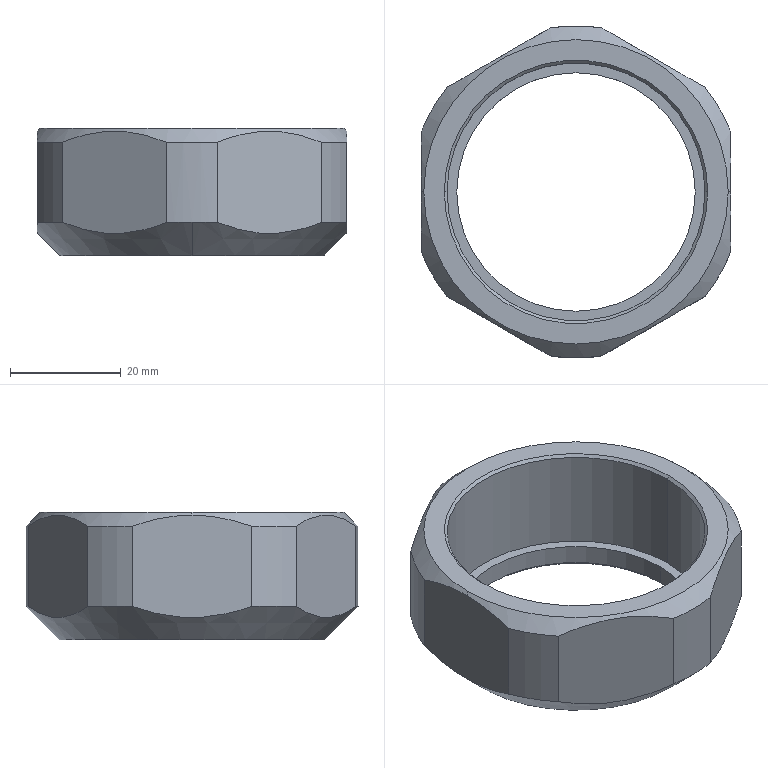Part | SolidWorks | features BaseBody 1 | 1 solid | 27 faces | box 56 x 60 x 23 mm | volume 20223 mm3 | cylinder 10 | plane 9 | cone 8 | commonest cylinder face diameters 60 x6 43.1 x2 46.6 x2
STEP:
#1=CARTESIAN_POINT('',(-23.3,0.,4.));
#2=VERTEX_POINT('',#1);
#3=CARTESIAN_POINT('',(23.3,0.,4.));
#4=VERTEX_POINT('',#3);
#5=CARTESIAN_POINT('',(0.,0.,4.));
#6=DIRECTION('',(0.,0.,1.));
#7=DIRECTION('',(1.,0.,0.));
#8=AXIS2_PLACEMENT_3D('',#5,#6,#7);
#9=CIRCLE('',#8,23.3);
#10=EDGE_CURVE('',#2,#4,#9,.T.);
#11=ORIENTED_EDGE('',*,*,#10,.F.);
#12=CARTESIAN_POINT('',(-23.3,0.,22.5));
#13=VERTEX_POINT('',#12);
#14=CARTESIAN_POINT('',(-23.3,0.,4.));
#15=DIRECTION('',(0.,0.,1.));
#16=VECTOR('',#15,1000.);
#17=LINE('',#14,#16);
#18=EDGE_CURVE('',#2,#13,#17,.T.);
#19=ORIENTED_EDGE('',*,*,#18,.T.);
#20=CARTESIAN_POINT('',(23.3,0.,22.5));
#21=VERTEX_POINT('',#20);
#22=CARTESIAN_POINT('',(0.,0.,22.5));
#23=DIRECTION('',(0.,0.,-1.));
#24=DIRECTION('',(1.,0.,0.));
#25=AXIS2_PLACEMENT_3D('',#22,#23,#24);
#26=CIRCLE('',#25,23.3);
#27=EDGE_CURVE('',#21,#13,#26,.T.);
#28=ORIENTED_EDGE('',*,*,#27,.F.);
#29=CARTESIAN_POINT('',(23.3,0.,4.));
#30=DIRECTION('',(0.,0.,1.));
#31=VECTOR('',#30,1000.);
#32=LINE('',#29,#31);
#33=EDGE_CURVE('',#4,#21,#32,.T.);
#34=ORIENTED_EDGE('',*,*,#33,.F.);
#35=EDGE_LOOP('',(#11,#19,#28,#34));
#36=FACE_OUTER_BOUND('',#35,.T.);
#37=CARTESIAN_POINT('',(0.,0.,4.));
#38=DIRECTION('',(0.,0.,1.));
#39=DIRECTION('',(1.,0.,0.));
#40=AXIS2_PLACEMENT_3D('',#37,#38,#39);
#41=CYLINDRICAL_SURFACE('',#40,23.3);
#42=ADVANCED_FACE('',(#36),#41,.F.);
#43=ORIENTED_EDGE('',*,*,#27,.T.);
#44=CARTESIAN_POINT('',(-23.8,0.,23.));
#45=VERTEX_POINT('',#44);
#46=CARTESIAN_POINT('',(-23.8,0.,23.));
#47=DIRECTION('',(-0.7071,0.,0.7071));
#48=VECTOR('',#47,1000.);
#49=LINE('',#46,#48);
#50=EDGE_CURVE('',#13,#45,#49,.T.);
#51=ORIENTED_EDGE('',*,*,#50,.T.);
#52=CARTESIAN_POINT('',(23.8,0.,23.));
#53=VERTEX_POINT('',#52);
#54=CARTESIAN_POINT('',(0.,0.,23.));
#55=DIRECTION('',(0.,0.,-1.));
#56=DIRECTION('',(1.,0.,0.));
#57=AXIS2_PLACEMENT_3D('',#54,#55,#56);
#58=CIRCLE('',#57,23.8);
#59=EDGE_CURVE('',#53,#45,#58,.T.);
#60=ORIENTED_EDGE('',*,*,#59,.F.);
#61=CARTESIAN_POINT('',(23.8,0.,23.));
#62=DIRECTION('',(0.7071,0.,0.7071));
#63=VECTOR('',#62,1000.);
#64=LINE('',#61,#63);
#65=EDGE_CURVE('',#21,#53,#64,.T.);
#66=ORIENTED_EDGE('',*,*,#65,.F.);
#67=EDGE_LOOP('',(#43,#51,#60,#66));
#68=FACE_OUTER_BOUND('',#67,.T.);
#69=CARTESIAN_POINT('',(0.,0.,23.));
#70=DIRECTION('',(0.,0.,1.));
#71=DIRECTION('',(1.,0.,0.));
#72=AXIS2_PLACEMENT_3D('',#69,#70,#71);
#73=CONICAL_SURFACE('',#72,23.8,0.7854);
#74=ADVANCED_FACE('',(#68),#73,.F.);
#75=CARTESIAN_POINT('',(21.55,0.,4.));
#76=VERTEX_POINT('',#75);
#77=CARTESIAN_POINT('',(-21.55,0.,4.));
#78=VERTEX_POINT('',#77);
#79=CARTESIAN_POINT('',(0.,0.,4.));
#80=DIRECTION('',(0.,0.,-1.));
#81=DIRECTION('',(-1.,0.,0.));
#82=AXIS2_PLACEMENT_3D('',#79,#80,#81);
#83=CIRCLE('',#82,21.55);
#84=EDGE_CURVE('',#76,#78,#83,.T.);
#85=ORIENTED_EDGE('',*,*,#84,.F.);
#86=CARTESIAN_POINT('',(21.55,0.,0.5));
#87=VERTEX_POINT('',#86);
#88=CARTESIAN_POINT('',(21.55,0.,23.));
#89=DIRECTION('',(0.,0.,-1.));
#90=VECTOR('',#89,1000.);
#91=LINE('',#88,#90);
#92=EDGE_CURVE('',#76,#87,#91,.T.);
#93=ORIENTED_EDGE('',*,*,#92,.T.);
#94=CARTESIAN_POINT('',(-21.55,0.,0.5));
#95=VERTEX_POINT('',#94);
#96=CARTESIAN_POINT('',(0.,0.,0.5));
#97=DIRECTION('',(0.,0.,1.));
#98=DIRECTION('',(-1.,0.,0.));
#99=AXIS2_PLACEMENT_3D('',#96,#97,#98);
#100=CIRCLE('',#99,21.55);
#101=EDGE_CURVE('',#95,#87,#100,.T.);
#102=ORIENTED_EDGE('',*,*,#101,.F.);
#103=CARTESIAN_POINT('',(-21.55,0.,23.));
#104=DIRECTION('',(0.,0.,-1.));
#105=VECTOR('',#104,1000.);
#106=LINE('',#103,#105);
#107=EDGE_CURVE('',#78,#95,#106,.T.);
#108=ORIENTED_EDGE('',*,*,#107,.F.);
#109=EDGE_LOOP('',(#85,#93,#102,#108));
#110=FACE_OUTER_BOUND('',#109,.T.);
#111=CARTESIAN_POINT('',(0.,0.,23.));
#112=DIRECTION('',(0.,0.,-1.));
#113=DIRECTION('',(-1.,0.,0.));
#114=AXIS2_PLACEMENT_3D('',#111,#112,#113);
#115=CYLINDRICAL_SURFACE('',#114,21.55);
#116=ADVANCED_FACE('',(#110),#115,.F.);
#117=ORIENTED_EDGE('',*,*,#101,.T.);
#118=CARTESIAN_POINT('',(22.05,0.,0.));
#119=VERTEX_POINT('',#118);
#120=CARTESIAN_POINT('',(22.05,0.,0.));
#121=DIRECTION('',(0.7071,0.,-0.7071));
#122=VECTOR('',#121,1000.);
#123=LINE('',#120,#122);
#124=EDGE_CURVE('',#87,#119,#123,.T.);
#125=ORIENTED_EDGE('',*,*,#124,.T.);
#126=CARTESIAN_POINT('',(-22.05,0.,0.));
#127=VERTEX_POINT('',#126);
#128=CARTESIAN_POINT('',(0.,0.,0.));
#129=DIRECTION('',(0.,0.,1.));
#130=DIRECTION('',(-1.,0.,0.));
#131=AXIS2_PLACEMENT_3D('',#128,#129,#130);
#132=CIRCLE('',#131,22.05);
#133=EDGE_CURVE('',#127,#119,#132,.T.);
#134=ORIENTED_EDGE('',*,*,#133,.F.);
#135=CARTESIAN_POINT('',(-22.05,0.,0.));
#136=DIRECTION('',(-0.7071,0.,-0.7071));
#137=VECTOR('',#136,1000.);
#138=LINE('',#135,#137);
#139=EDGE_CURVE('',#95,#127,#138,.T.);
#140=ORIENTED_EDGE('',*,*,#139,.F.);
#141=EDGE_LOOP('',(#117,#125,#134,#140));
#142=FACE_OUTER_BOUND('',#141,.T.);
#143=CARTESIAN_POINT('',(0.,0.,0.));
#144=DIRECTION('',(0.,0.,-1.));
#145=DIRECTION('',(-1.,0.,0.));
#146=AXIS2_PLACEMENT_3D('',#143,#144,#145);
#147=CONICAL_SURFACE('',#146,22.05,0.7854);
#148=ADVANCED_FACE('',(#142),#147,.F.);
#149=CARTESIAN_POINT('',(27.5,0.,23.));
#150=VERTEX_POINT('',#149);
#151=CARTESIAN_POINT('',(-27.5,0.,23.));
#152=VERTEX_POINT('',#151);
#153=CARTESIAN_POINT('',(0.,0.,23.));
#154=DIRECTION('',(0.,0.,1.));
#155=DIRECTION('',(-1.,0.,0.));
#156=AXIS2_PLACEMENT_3D('',#153,#154,#155);
#157=CIRCLE('',#156,27.5);
#158=EDGE_CURVE('',#150,#152,#157,.T.);
#159=ORIENTED_EDGE('',*,*,#158,.F.);
#160=CARTESIAN_POINT('',(28.,0.,22.5));
#161=VERTEX_POINT('',#160);
#162=CARTESIAN_POINT('',(30.,0.,20.5));
#163=DIRECTION('',(0.7071,0.,-0.7071));
#164=VECTOR('',#163,1000.);
#165=LINE('',#162,#164);
#166=EDGE_CURVE('',#150,#161,#165,.T.);
#167=ORIENTED_EDGE('',*,*,#166,.T.);
#168=CARTESIAN_POINT('',(28.,10.77,20.5));
#169=VERTEX_POINT('',#168);
#170=CARTESIAN_POINT('',(28.,0.,22.5));
#171=CARTESIAN_POINT('',(28.,1.857,22.5));
#172=CARTESIAN_POINT('',(28.,3.679,22.314));
#173=CARTESIAN_POINT('',(28.,7.266,21.626));
#174=CARTESIAN_POINT('',(28.,9.029,21.125));
#175=CARTESIAN_POINT('',(28.,10.77,20.5));
#176=B_SPLINE_CURVE_WITH_KNOTS('',3,(#170,#171,#172,#173,#174,#175),.UNSPECIFIED.,.F.,.F.,(4,2,4),(0.,0.005477,0.01095),.UNSPECIFIED.);
#177=EDGE_CURVE('',#161,#169,#176,.T.);
#178=ORIENTED_EDGE('',*,*,#177,.T.);
#179=CARTESIAN_POINT('',(23.327,18.864,20.5));
#180=VERTEX_POINT('',#179);
#181=CARTESIAN_POINT('',(0.,0.,20.5));
#182=DIRECTION('',(0.,0.,1.));
#183=DIRECTION('',(-1.,0.,0.));
#184=AXIS2_PLACEMENT_3D('',#181,#182,#183);
#185=CIRCLE('',#184,30.);
#186=EDGE_CURVE('',#169,#180,#185,.T.);
#187=ORIENTED_EDGE('',*,*,#186,.T.);
#188=CARTESIAN_POINT('',(4.673,29.634,20.5));
#189=VERTEX_POINT('',#188);
#190=CARTESIAN_POINT('',(23.327,18.864,20.5));
#191=CARTESIAN_POINT('',(21.82,19.734,21.125));
#192=CARTESIAN_POINT('',(20.292,20.616,21.626));
#193=CARTESIAN_POINT('',(17.186,22.409,22.314));
#194=CARTESIAN_POINT('',(15.608,23.32,22.5));
#195=CARTESIAN_POINT('',(12.392,25.177,22.5));
#196=CARTESIAN_POINT('',(10.813,26.088,22.314));
#197=CARTESIAN_POINT('',(7.708,27.882,21.626));
#198=CARTESIAN_POINT('',(6.18,28.763,21.125));
#199=CARTESIAN_POINT('',(4.673,29.634,20.5));
#200=B_SPLINE_CURVE_WITH_KNOTS('',3,(#190,#191,#192,#193,#194,#195,#196,#197,#198,#199),.UNSPECIFIED.,.F.,.F.,(4,2,2,2,4),(-0.01095,-0.005472,0.000005126,0.005482,0.01096),.UNSPECIFIED.);
#201=EDGE_CURVE('',#180,#189,#200,.T.);
#202=ORIENTED_EDGE('',*,*,#201,.T.);
#203=CARTESIAN_POINT('',(-4.673,29.634,20.5));
#204=VERTEX_POINT('',#203);
#205=CARTESIAN_POINT('',(0.,0.,20.5));
#206=DIRECTION('',(0.,0.,1.));
#207=DIRECTION('',(-1.,0.,0.));
#208=AXIS2_PLACEMENT_3D('',#205,#206,#207);
#209=CIRCLE('',#208,30.);
#210=EDGE_CURVE('',#189,#204,#209,.T.);
#211=ORIENTED_EDGE('',*,*,#210,.T.);
#212=CARTESIAN_POINT('',(-23.327,18.864,20.5));
#213=VERTEX_POINT('',#212);
#214=CARTESIAN_POINT('',(-4.673,29.634,20.5));
#215=CARTESIAN_POINT('',(-6.18,28.763,21.125));
#216=CARTESIAN_POINT('',(-7.708,27.881,21.626));
#217=CARTESIAN_POINT('',(-10.814,26.088,22.314));
#218=CARTESIAN_POINT('',(-12.392,25.177,22.5));
#219=CARTESIAN_POINT('',(-15.608,23.32,22.5));
#220=CARTESIAN_POINT('',(-17.187,22.409,22.314));
#221=CARTESIAN_POINT('',(-20.292,20.616,21.626));
#222=CARTESIAN_POINT('',(-21.82,19.734,21.125));
#223=CARTESIAN_POINT('',(-23.327,18.864,20.5));
#224=B_SPLINE_CURVE_WITH_KNOTS('',3,(#214,#215,#216,#217,#218,#219,#220,#221,#222,#223),.UNSPECIFIED.,.F.,.F.,(4,2,2,2,4),(-0.01095,-0.005472,0.000005126,0.005482,0.01096),.UNSPECIFIED.);
#225=EDGE_CURVE('',#204,#213,#224,.T.);
#226=ORIENTED_EDGE('',*,*,#225,.T.);
#227=CARTESIAN_POINT('',(-28.,10.77,20.5));
#228=VERTEX_POINT('',#227);
#229=CARTESIAN_POINT('',(0.,0.,20.5));
#230=DIRECTION('',(0.,0.,1.));
#231=DIRECTION('',(-1.,0.,0.));
#232=AXIS2_PLACEMENT_3D('',#229,#230,#231);
#233=CIRCLE('',#232,30.);
#234=EDGE_CURVE('',#213,#228,#233,.T.);
#235=ORIENTED_EDGE('',*,*,#234,.T.);
#236=CARTESIAN_POINT('',(-28.,0.,22.5));
#237=VERTEX_POINT('',#236);
#238=CARTESIAN_POINT('',(-28.,10.77,20.5));
#239=CARTESIAN_POINT('',(-28.,9.029,21.125));
#240=CARTESIAN_POINT('',(-28.,7.266,21.626));
#241=CARTESIAN_POINT('',(-28.,3.679,22.314));
#242=CARTESIAN_POINT('',(-28.,1.857,22.5));
#243=CARTESIAN_POINT('',(-28.,0.,22.5));
#244=B_SPLINE_CURVE_WITH_KNOTS('',3,(#238,#239,#240,#241,#242,#243),.UNSPECIFIED.,.F.,.F.,(4,2,4),(0.,0.005477,0.01095),.UNSPECIFIED.);
#245=EDGE_CURVE('',#228,#237,#244,.T.);
#246=ORIENTED_EDGE('',*,*,#245,.T.);
#247=CARTESIAN_POINT('',(-30.,0.,20.5));
#248=DIRECTION('',(-0.7071,0.,-0.7071));
#249=VECTOR('',#248,1000.);
#250=LINE('',#247,#249);
#251=EDGE_CURVE('',#152,#237,#250,.T.);
#252=ORIENTED_EDGE('',*,*,#251,.F.);
#253=EDGE_LOOP('',(#159,#167,#178,#187,#202,#211,#226,#235,#246,#252));
#254=FACE_OUTER_BOUND('',#253,.T.);
#255=CARTESIAN_POINT('',(0.,0.,20.5));
#256=DIRECTION('',(0.,0.,-1.));
#257=DIRECTION('',(-1.,0.,0.));
#258=AXIS2_PLACEMENT_3D('',#255,#256,#257);
#259=CONICAL_SURFACE('',#258,30.,0.7854);
#260=ADVANCED_FACE('',(#254),#259,.T.);
#261=CARTESIAN_POINT('',(0.,-24.,0.));
#262=VERTEX_POINT('',#261);
#263=CARTESIAN_POINT('',(0.,24.,0.));
#264=VERTEX_POINT('',#263);
#265=CARTESIAN_POINT('',(0.,0.,0.));
#266=DIRECTION('',(0.,0.,1.));
#267=DIRECTION('',(0.,-1.,0.));
#268=AXIS2_PLACEMENT_3D('',#265,#266,#267);
#269=CIRCLE('',#268,24.);
#270=EDGE_CURVE('',#262,#264,#269,.T.);
#271=ORIENTED_EDGE('',*,*,#270,.T.);
#272=CARTESIAN_POINT('',(0.,30.,6.));
#273=VERTEX_POINT('',#272);
#274=CARTESIAN_POINT('',(0.,30.,6.));
#275=DIRECTION('',(0.,0.7071,0.7071));
#276=VECTOR('',#275,1000.);
#277=LINE('',#274,#276);
#278=EDGE_CURVE('',#264,#273,#277,.T.);
#279=ORIENTED_EDGE('',*,*,#278,.T.);
#280=CARTESIAN_POINT('',(4.673,29.634,6.));
#281=VERTEX_POINT('',#280);
#282=CARTESIAN_POINT('',(0.,0.,6.));
#283=DIRECTION('',(0.,0.,1.));
#284=DIRECTION('',(-1.,0.,0.));
#285=AXIS2_PLACEMENT_3D('',#282,#283,#284);
#286=CIRCLE('',#285,30.);
#287=EDGE_CURVE('',#281,#273,#286,.T.);
#288=ORIENTED_EDGE('',*,*,#287,.F.);
#289=CARTESIAN_POINT('',(23.327,18.864,6.));
#290=VERTEX_POINT('',#289);
#291=CARTESIAN_POINT('',(4.673,29.634,6.));
#292=CARTESIAN_POINT('',(6.18,28.763,5.375));
#293=CARTESIAN_POINT('',(7.708,27.882,4.874));
#294=CARTESIAN_POINT('',(10.813,26.088,4.186));
#295=CARTESIAN_POINT('',(12.392,25.177,4.));
#296=CARTESIAN_POINT('',(15.608,23.32,4.));
#297=CARTESIAN_POINT('',(17.186,22.409,4.186));
#298=CARTESIAN_POINT('',(20.292,20.616,4.874));
#299=CARTESIAN_POINT('',(21.82,19.734,5.375));
#300=CARTESIAN_POINT('',(23.327,18.864,6.));
#301=B_SPLINE_CURVE_WITH_KNOTS('',3,(#291,#292,#293,#294,#295,#296,#297,#298,#299,#300),.UNSPECIFIED.,.F.,.F.,(4,2,2,2,4),(-0.01096,-0.005482,-0.000005126,0.005472,0.01095),.UNSPECIFIED.);
#302=EDGE_CURVE('',#281,#290,#301,.T.);
#303=ORIENTED_EDGE('',*,*,#302,.T.);
#304=CARTESIAN_POINT('',(28.,10.77,6.));
#305=VERTEX_POINT('',#304);
#306=CARTESIAN_POINT('',(0.,0.,6.));
#307=DIRECTION('',(0.,0.,1.));
#308=DIRECTION('',(-1.,0.,0.));
#309=AXIS2_PLACEMENT_3D('',#306,#307,#308);
#310=CIRCLE('',#309,30.);
#311=EDGE_CURVE('',#305,#290,#310,.T.);
#312=ORIENTED_EDGE('',*,*,#311,.F.);
#313=CARTESIAN_POINT('',(28.,-10.77,6.));
#314=VERTEX_POINT('',#313);
#315=CARTESIAN_POINT('',(28.,10.77,6.));
#316=CARTESIAN_POINT('',(28.,9.029,5.375));
#317=CARTESIAN_POINT('',(28.,7.266,4.874));
#318=CARTESIAN_POINT('',(28.,3.679,4.186));
#319=CARTESIAN_POINT('',(28.,1.857,4.));
#320=CARTESIAN_POINT('',(28.,-1.857,4.));
#321=CARTESIAN_POINT('',(28.,-3.679,4.186));
#322=CARTESIAN_POINT('',(28.,-7.266,4.874));
#323=CARTESIAN_POINT('',(28.,-9.029,5.375));
#324=CARTESIAN_POINT('',(28.,-10.77,6.));
#325=B_SPLINE_CURVE_WITH_KNOTS('',3,(#315,#316,#317,#318,#319,#320,#321,#322,#323,#324),.UNSPECIFIED.,.F.,.F.,(4,2,2,2,4),(-0.01095,-0.005477,0.,0.005477,0.01095),.UNSPECIFIED.);
#326=EDGE_CURVE('',#305,#314,#325,.T.);
#327=ORIENTED_EDGE('',*,*,#326,.T.);
#328=CARTESIAN_POINT('',(23.327,-18.864,6.));
#329=VERTEX_POINT('',#328);
#330=CARTESIAN_POINT('',(0.,0.,6.));
#331=DIRECTION('',(0.,0.,1.));
#332=DIRECTION('',(-1.,0.,0.));
#333=AXIS2_PLACEMENT_3D('',#330,#331,#332);
#334=CIRCLE('',#333,30.);
#335=EDGE_CURVE('',#329,#314,#334,.T.);
#336=ORIENTED_EDGE('',*,*,#335,.F.);
#337=CARTESIAN_POINT('',(4.673,-29.634,6.));
#338=VERTEX_POINT('',#337);
#339=CARTESIAN_POINT('',(23.327,-18.864,6.));
#340=CARTESIAN_POINT('',(21.82,-19.734,5.375));
#341=CARTESIAN_POINT('',(20.292,-20.616,4.874));
#342=CARTESIAN_POINT('',(17.187,-22.409,4.186));
#343=CARTESIAN_POINT('',(15.608,-23.32,4.));
#344=CARTESIAN_POINT('',(12.392,-25.177,4.));
#345=CARTESIAN_POINT('',(10.814,-26.088,4.186));
#346=CARTESIAN_POINT('',(7.708,-27.881,4.874));
#347=CARTESIAN_POINT('',(6.18,-28.763,5.375));
#348=CARTESIAN_POINT('',(4.673,-29.634,6.));
#349=B_SPLINE_CURVE_WITH_KNOTS('',3,(#339,#340,#341,#342,#343,#344,#345,#346,#347,#348),.UNSPECIFIED.,.F.,.F.,(4,2,2,2,4),(-0.01096,-0.005482,-0.000005126,0.005472,0.01095),.UNSPECIFIED.);
#350=EDGE_CURVE('',#329,#338,#349,.T.);
#351=ORIENTED_EDGE('',*,*,#350,.T.);
#352=CARTESIAN_POINT('',(0.,-30.,6.));
#353=VERTEX_POINT('',#352);
#354=CARTESIAN_POINT('',(0.,0.,6.));
#355=DIRECTION('',(0.,0.,1.));
#356=DIRECTION('',(-1.,0.,0.));
#357=AXIS2_PLACEMENT_3D('',#354,#355,#356);
#358=CIRCLE('',#357,30.);
#359=EDGE_CURVE('',#353,#338,#358,.T.);
#360=ORIENTED_EDGE('',*,*,#359,.F.);
#361=CARTESIAN_POINT('',(0.,-30.,6.));
#362=DIRECTION('',(0.,-0.7071,0.7071));
#363=VECTOR('',#362,1000.);
#364=LINE('',#361,#363);
#365=EDGE_CURVE('',#262,#353,#364,.T.);
#366=ORIENTED_EDGE('',*,*,#365,.F.);
#367=EDGE_LOOP('',(#271,#279,#288,#303,#312,#327,#336,#351,#360,#366));
#368=FACE_OUTER_BOUND('',#367,.T.);
#369=CARTESIAN_POINT('',(0.,0.,6.));
#370=DIRECTION('',(0.,0.,1.));
#371=DIRECTION('',(0.,-1.,0.));
#372=AXIS2_PLACEMENT_3D('',#369,#370,#371);
#373=CONICAL_SURFACE('',#372,30.,0.7854);
#374=ADVANCED_FACE('',(#368),#373,.T.);
#375=ORIENTED_EDGE('',*,*,#18,.F.);
#376=CARTESIAN_POINT('',(0.,0.,4.));
#377=DIRECTION('',(0.,0.,1.));
#378=DIRECTION('',(1.,0.,0.));
#379=AXIS2_PLACEMENT_3D('',#376,#377,#378);
#380=CIRCLE('',#379,23.3);
#381=EDGE_CURVE('',#4,#2,#380,.T.);
#382=ORIENTED_EDGE('',*,*,#381,.F.);
#383=ORIENTED_EDGE('',*,*,#33,.T.);
#384=CARTESIAN_POINT('',(0.,0.,22.5));
#385=DIRECTION('',(0.,0.,-1.));
#386=DIRECTION('',(1.,0.,0.));
#387=AXIS2_PLACEMENT_3D('',#384,#385,#386);
#388=CIRCLE('',#387,23.3);
#389=EDGE_CURVE('',#13,#21,#388,.T.);
#390=ORIENTED_EDGE('',*,*,#389,.F.);
#391=EDGE_LOOP('',(#375,#382,#383,#390));
#392=FACE_OUTER_BOUND('',#391,.T.);
#393=CARTESIAN_POINT('',(0.,0.,4.));
#394=DIRECTION('',(0.,0.,1.));
#395=DIRECTION('',(1.,0.,0.));
#396=AXIS2_PLACEMENT_3D('',#393,#394,#395);
#397=CYLINDRICAL_SURFACE('',#396,23.3);
#398=ADVANCED_FACE('',(#392),#397,.F.);
#399=CARTESIAN_POINT('',(0.,0.,4.));
#400=DIRECTION('',(0.,0.,-1.));
#401=DIRECTION('',(-1.,0.,0.));
#402=AXIS2_PLACEMENT_3D('',#399,#400,#401);
#403=CIRCLE('',#402,21.55);
#404=EDGE_CURVE('',#78,#76,#403,.T.);
#405=ORIENTED_EDGE('',*,*,#404,.T.);
#406=ORIENTED_EDGE('',*,*,#84,.T.);
#407=EDGE_LOOP('',(#405,#406));
#408=FACE_BOUND('',#407,.T.);
#409=ORIENTED_EDGE('',*,*,#381,.T.);
#410=ORIENTED_EDGE('',*,*,#10,.T.);
#411=EDGE_LOOP('',(#409,#410));
#412=FACE_OUTER_BOUND('',#411,.T.);
#413=CARTESIAN_POINT('',(0.,0.,4.));
#414=DIRECTION('',(0.,0.,1.));
#415=DIRECTION('',(1.,0.,0.));
#416=AXIS2_PLACEMENT_3D('',#413,#414,#415);
#417=PLANE('',#416);
#418=ADVANCED_FACE('',(#408,#412),#417,.T.);
#419=ORIENTED_EDGE('',*,*,#50,.F.);
#420=ORIENTED_EDGE('',*,*,#389,.T.);
#421=ORIENTED_EDGE('',*,*,#65,.T.);
#422=CARTESIAN_POINT('',(0.,0.,23.));
#423=DIRECTION('',(0.,0.,-1.));
#424=DIRECTION('',(1.,0.,0.));
#425=AXIS2_PLACEMENT_3D('',#422,#423,#424);
#426=CIRCLE('',#425,23.8);
#427=EDGE_CURVE('',#45,#53,#426,.T.);
#428=ORIENTED_EDGE('',*,*,#427,.F.);
#429=EDGE_LOOP('',(#419,#420,#421,#428));
#430=FACE_OUTER_BOUND('',#429,.T.);
#431=CARTESIAN_POINT('',(0.,0.,23.));
#432=DIRECTION('',(0.,0.,1.));
#433=DIRECTION('',(1.,0.,0.));
#434=AXIS2_PLACEMENT_3D('',#431,#432,#433);
#435=CONICAL_SURFACE('',#434,23.8,0.7854);
#436=ADVANCED_FACE('',(#430),#435,.F.);
#437=ORIENTED_EDGE('',*,*,#92,.F.);
#438=ORIENTED_EDGE('',*,*,#404,.F.);
#439=ORIENTED_EDGE('',*,*,#107,.T.);
#440=CARTESIAN_POINT('',(0.,0.,0.5));
#441=DIRECTION('',(0.,0.,1.));
#442=DIRECTION('',(-1.,0.,0.));
#443=AXIS2_PLACEMENT_3D('',#440,#441,#442);
#444=CIRCLE('',#443,21.55);
#445=EDGE_CURVE('',#87,#95,#444,.T.);
#446=ORIENTED_EDGE('',*,*,#445,.F.);
#447=EDGE_LOOP('',(#437,#438,#439,#446));
#448=FACE_OUTER_BOUND('',#447,.T.);
#449=CARTESIAN_POINT('',(0.,0.,23.));
#450=DIRECTION('',(0.,0.,-1.));
#451=DIRECTION('',(-1.,0.,0.));
#452=AXIS2_PLACEMENT_3D('',#449,#450,#451);
#453=CYLINDRICAL_SURFACE('',#452,21.55);
#454=ADVANCED_FACE('',(#448),#453,.F.);
#455=ORIENTED_EDGE('',*,*,#59,.T.);
#456=ORIENTED_EDGE('',*,*,#427,.T.);
#457=EDGE_LOOP('',(#455,#456));
#458=FACE_BOUND('',#457,.T.);
#459=CARTESIAN_POINT('',(0.,0.,23.));
#460=DIRECTION('',(0.,0.,1.));
#461=DIRECTION('',(-1.,0.,0.));
#462=AXIS2_PLACEMENT_3D('',#459,#460,#461);
#463=CIRCLE('',#462,27.5);
#464=EDGE_CURVE('',#152,#150,#463,.T.);
#465=ORIENTED_EDGE('',*,*,#464,.T.);
#466=ORIENTED_EDGE('',*,*,#158,.T.);
#467=EDGE_LOOP('',(#465,#466));
#468=FACE_OUTER_BOUND('',#467,.T.);
#469=CARTESIAN_POINT('',(0.,0.,23.));
#470=DIRECTION('',(0.,0.,1.));
#471=DIRECTION('',(1.,0.,0.));
#472=AXIS2_PLACEMENT_3D('',#469,#470,#471);
#473=PLANE('',#472);
#474=ADVANCED_FACE('',(#458,#468),#473,.T.);
#475=ORIENTED_EDGE('',*,*,#124,.F.);
#476=ORIENTED_EDGE('',*,*,#445,.T.);
#477=ORIENTED_EDGE('',*,*,#139,.T.);
#478=CARTESIAN_POINT('',(0.,0.,0.));
#479=DIRECTION('',(0.,0.,1.));
#480=DIRECTION('',(-1.,0.,0.));
#481=AXIS2_PLACEMENT_3D('',#478,#479,#480);
#482=CIRCLE('',#481,22.05);
#483=EDGE_CURVE('',#119,#127,#482,.T.);
#484=ORIENTED_EDGE('',*,*,#483,.F.);
#485=EDGE_LOOP('',(#475,#476,#477,#484));
#486=FACE_OUTER_BOUND('',#485,.T.);
#487=CARTESIAN_POINT('',(0.,0.,0.));
#488=DIRECTION('',(0.,0.,-1.));
#489=DIRECTION('',(-1.,0.,0.));
#490=AXIS2_PLACEMENT_3D('',#487,#488,#489);
#491=CONICAL_SURFACE('',#490,22.05,0.7854);
#492=ADVANCED_FACE('',(#486),#491,.F.);
#493=ORIENTED_EDGE('',*,*,#166,.F.);
#494=ORIENTED_EDGE('',*,*,#464,.F.);
#495=ORIENTED_EDGE('',*,*,#251,.T.);
#496=CARTESIAN_POINT('',(-28.,-10.77,20.5));
#497=VERTEX_POINT('',#496);
#498=CARTESIAN_POINT('',(-28.,0.,22.5));
#499=CARTESIAN_POINT('',(-28.,-1.857,22.5));
#500=CARTESIAN_POINT('',(-28.,-3.679,22.314));
#501=CARTESIAN_POINT('',(-28.,-7.266,21.626));
#502=CARTESIAN_POINT('',(-28.,-9.029,21.125));
#503=CARTESIAN_POINT('',(-28.,-10.77,20.5));
#504=B_SPLINE_CURVE_WITH_KNOTS('',3,(#498,#499,#500,#501,#502,#503),.UNSPECIFIED.,.F.,.F.,(4,2,4),(0.01095,0.01643,0.02191),.UNSPECIFIED.);
#505=EDGE_CURVE('',#237,#497,#504,.T.);
#506=ORIENTED_EDGE('',*,*,#505,.T.);
#507=CARTESIAN_POINT('',(-23.327,-18.864,20.5));
#508=VERTEX_POINT('',#507);
#509=CARTESIAN_POINT('',(0.,0.,20.5));
#510=DIRECTION('',(0.,0.,1.));
#511=DIRECTION('',(1.,0.,0.));
#512=AXIS2_PLACEMENT_3D('',#509,#510,#511);
#513=CIRCLE('',#512,30.);
#514=EDGE_CURVE('',#497,#508,#513,.T.);
#515=ORIENTED_EDGE('',*,*,#514,.T.);
#516=CARTESIAN_POINT('',(-4.673,-29.634,20.5));
#517=VERTEX_POINT('',#516);
#518=CARTESIAN_POINT('',(-23.327,-18.864,20.5));
#519=CARTESIAN_POINT('',(-21.82,-19.734,21.125));
#520=CARTESIAN_POINT('',(-20.292,-20.616,21.626));
#521=CARTESIAN_POINT('',(-17.186,-22.409,22.314));
#522=CARTESIAN_POINT('',(-15.608,-23.32,22.5));
#523=CARTESIAN_POINT('',(-12.392,-25.177,22.5));
#524=CARTESIAN_POINT('',(-10.813,-26.088,22.314));
#525=CARTESIAN_POINT('',(-7.708,-27.882,21.626));
#526=CARTESIAN_POINT('',(-6.18,-28.763,21.125));
#527=CARTESIAN_POINT('',(-4.673,-29.634,20.5));
#528=B_SPLINE_CURVE_WITH_KNOTS('',3,(#518,#519,#520,#521,#522,#523,#524,#525,#526,#527),.UNSPECIFIED.,.F.,.F.,(4,2,2,2,4),(-0.01095,-0.005472,0.000005126,0.005482,0.01096),.UNSPECIFIED.);
#529=EDGE_CURVE('',#508,#517,#528,.T.);
#530=ORIENTED_EDGE('',*,*,#529,.T.);
#531=CARTESIAN_POINT('',(4.673,-29.634,20.5));
#532=VERTEX_POINT('',#531);
#533=CARTESIAN_POINT('',(0.,0.,20.5));
#534=DIRECTION('',(0.,0.,1.));
#535=DIRECTION('',(1.,0.,0.));
#536=AXIS2_PLACEMENT_3D('',#533,#534,#535);
#537=CIRCLE('',#536,30.);
#538=EDGE_CURVE('',#517,#532,#537,.T.);
#539=ORIENTED_EDGE('',*,*,#538,.T.);
#540=CARTESIAN_POINT('',(23.327,-18.864,20.5));
#541=VERTEX_POINT('',#540);
#542=CARTESIAN_POINT('',(4.673,-29.634,20.5));
#543=CARTESIAN_POINT('',(6.18,-28.763,21.125));
#544=CARTESIAN_POINT('',(7.708,-27.881,21.626));
#545=CARTESIAN_POINT('',(10.814,-26.088,22.314));
#546=CARTESIAN_POINT('',(12.392,-25.177,22.5));
#547=CARTESIAN_POINT('',(15.608,-23.32,22.5));
#548=CARTESIAN_POINT('',(17.187,-22.409,22.314));
#549=CARTESIAN_POINT('',(20.292,-20.616,21.626));
#550=CARTESIAN_POINT('',(21.82,-19.734,21.125));
#551=CARTESIAN_POINT('',(23.327,-18.864,20.5));
#552=B_SPLINE_CURVE_WITH_KNOTS('',3,(#542,#543,#544,#545,#546,#547,#548,#549,#550,#551),.UNSPECIFIED.,.F.,.F.,(4,2,2,2,4),(-0.01095,-0.005472,0.000005126,0.005482,0.01096),.UNSPECIFIED.);
#553=EDGE_CURVE('',#532,#541,#552,.T.);
#554=ORIENTED_EDGE('',*,*,#553,.T.);
#555=CARTESIAN_POINT('',(28.,-10.77,20.5));
#556=VERTEX_POINT('',#555);
#557=CARTESIAN_POINT('',(0.,0.,20.5));
#558=DIRECTION('',(0.,0.,1.));
#559=DIRECTION('',(1.,0.,0.));
#560=AXIS2_PLACEMENT_3D('',#557,#558,#559);
#561=CIRCLE('',#560,30.);
#562=EDGE_CURVE('',#541,#556,#561,.T.);
#563=ORIENTED_EDGE('',*,*,#562,.T.);
#564=CARTESIAN_POINT('',(28.,-10.77,20.5));
#565=CARTESIAN_POINT('',(28.,-9.029,21.125));
#566=CARTESIAN_POINT('',(28.,-7.266,21.626));
#567=CARTESIAN_POINT('',(28.,-3.679,22.314));
#568=CARTESIAN_POINT('',(28.,-1.857,22.5));
#569=CARTESIAN_POINT('',(28.,0.,22.5));
#570=B_SPLINE_CURVE_WITH_KNOTS('',3,(#564,#565,#566,#567,#568,#569),.UNSPECIFIED.,.F.,.F.,(4,2,4),(-0.01095,-0.005477,0.),.UNSPECIFIED.);
#571=EDGE_CURVE('',#556,#161,#570,.T.);
#572=ORIENTED_EDGE('',*,*,#571,.T.);
#573=EDGE_LOOP('',(#493,#494,#495,#506,#515,#530,#539,#554,#563,#572));
#574=FACE_OUTER_BOUND('',#573,.T.);
#575=CARTESIAN_POINT('',(0.,0.,20.5));
#576=DIRECTION('',(0.,0.,-1.));
#577=DIRECTION('',(-1.,0.,0.));
#578=AXIS2_PLACEMENT_3D('',#575,#576,#577);
#579=CONICAL_SURFACE('',#578,30.,0.7854);
#580=ADVANCED_FACE('',(#574),#579,.T.);
#581=ORIENTED_EDGE('',*,*,#133,.T.);
#582=ORIENTED_EDGE('',*,*,#483,.T.);
#583=EDGE_LOOP('',(#581,#582));
#584=FACE_BOUND('',#583,.T.);
#585=ORIENTED_EDGE('',*,*,#270,.F.);
#586=CARTESIAN_POINT('',(0.,0.,0.));
#587=DIRECTION('',(0.,0.,1.));
#588=DIRECTION('',(0.,-1.,0.));
#589=AXIS2_PLACEMENT_3D('',#586,#587,#588);
#590=CIRCLE('',#589,24.);
#591=EDGE_CURVE('',#264,#262,#590,.T.);
#592=ORIENTED_EDGE('',*,*,#591,.F.);
#593=EDGE_LOOP('',(#585,#592));
#594=FACE_OUTER_BOUND('',#593,.T.);
#595=CARTESIAN_POINT('',(0.,0.,0.));
#596=DIRECTION('',(0.,0.,1.));
#597=DIRECTION('',(1.,0.,0.));
#598=AXIS2_PLACEMENT_3D('',#595,#596,#597);
#599=PLANE('',#598);
#600=ADVANCED_FACE('',(#584,#594),#599,.F.);
#601=CARTESIAN_POINT('',(-28.,10.77,6.));
#602=VERTEX_POINT('',#601);
#603=CARTESIAN_POINT('',(-28.,10.77,23.));
#604=DIRECTION('',(0.,0.,1.));
#605=VECTOR('',#604,1000.);
#606=LINE('',#603,#605);
#607=EDGE_CURVE('',#602,#228,#606,.T.);
#608=ORIENTED_EDGE('',*,*,#607,.F.);
#609=CARTESIAN_POINT('',(-28.,-10.77,6.));
#610=VERTEX_POINT('',#609);
#611=CARTESIAN_POINT('',(-28.,-10.77,6.));
#612=CARTESIAN_POINT('',(-28.,-9.029,5.375));
#613=CARTESIAN_POINT('',(-28.,-7.266,4.874));
#614=CARTESIAN_POINT('',(-28.,-3.679,4.186));
#615=CARTESIAN_POINT('',(-28.,-1.857,4.));
#616=CARTESIAN_POINT('',(-28.,1.857,4.));
#617=CARTESIAN_POINT('',(-28.,3.679,4.186));
#618=CARTESIAN_POINT('',(-28.,7.266,4.874));
#619=CARTESIAN_POINT('',(-28.,9.029,5.375));
#620=CARTESIAN_POINT('',(-28.,10.77,6.));
#621=B_SPLINE_CURVE_WITH_KNOTS('',3,(#611,#612,#613,#614,#615,#616,#617,#618,#619,#620),.UNSPECIFIED.,.F.,.F.,(4,2,2,2,4),(-0.01095,-0.005477,0.,0.005477,0.01095),.UNSPECIFIED.);
#622=EDGE_CURVE('',#610,#602,#621,.T.);
#623=ORIENTED_EDGE('',*,*,#622,.F.);
#624=CARTESIAN_POINT('',(-28.,-10.77,23.));
#625=DIRECTION('',(0.,0.,-1.));
#626=VECTOR('',#625,1000.);
#627=LINE('',#624,#626);
#628=EDGE_CURVE('',#497,#610,#627,.T.);
#629=ORIENTED_EDGE('',*,*,#628,.F.);
#630=ORIENTED_EDGE('',*,*,#505,.F.);
#631=ORIENTED_EDGE('',*,*,#245,.F.);
#632=EDGE_LOOP('',(#608,#623,#629,#630,#631));
#633=FACE_OUTER_BOUND('',#632,.T.);
#634=CARTESIAN_POINT('',(-28.,10.77,23.));
#635=DIRECTION('',(1.,0.,0.));
#636=DIRECTION('',(0.,0.,-1.));
#637=AXIS2_PLACEMENT_3D('',#634,#635,#636);
#638=PLANE('',#637);
#639=ADVANCED_FACE('',(#633),#638,.F.);
#640=CARTESIAN_POINT('',(-23.327,18.864,6.));
#641=VERTEX_POINT('',#640);
#642=CARTESIAN_POINT('',(0.,0.,6.));
#643=DIRECTION('',(0.,0.,1.));
#644=DIRECTION('',(-1.,0.,0.));
#645=AXIS2_PLACEMENT_3D('',#642,#643,#644);
#646=CIRCLE('',#645,30.);
#647=EDGE_CURVE('',#641,#602,#646,.T.);
#648=ORIENTED_EDGE('',*,*,#647,.T.);
#649=ORIENTED_EDGE('',*,*,#607,.T.);
#650=ORIENTED_EDGE('',*,*,#234,.F.);
#651=CARTESIAN_POINT('',(-23.327,18.864,23.));
#652=DIRECTION('',(0.,0.,-1.));
#653=VECTOR('',#652,1000.);
#654=LINE('',#651,#653);
#655=EDGE_CURVE('',#213,#641,#654,.T.);
#656=ORIENTED_EDGE('',*,*,#655,.T.);
#657=EDGE_LOOP('',(#648,#649,#650,#656));
#658=FACE_OUTER_BOUND('',#657,.T.);
#659=CARTESIAN_POINT('',(0.,0.,23.));
#660=DIRECTION('',(0.,0.,-1.));
#661=DIRECTION('',(-1.,0.,0.));
#662=AXIS2_PLACEMENT_3D('',#659,#660,#661);
#663=CYLINDRICAL_SURFACE('',#662,30.);
#664=ADVANCED_FACE('',(#658),#663,.T.);
#665=ORIENTED_EDGE('',*,*,#225,.F.);
#666=CARTESIAN_POINT('',(-4.673,29.634,6.));
#667=VERTEX_POINT('',#666);
#668=CARTESIAN_POINT('',(-4.673,29.634,23.));
#669=DIRECTION('',(0.,0.,1.));
#670=VECTOR('',#669,1000.);
#671=LINE('',#668,#670);
#672=EDGE_CURVE('',#667,#204,#671,.T.);
#673=ORIENTED_EDGE('',*,*,#672,.F.);
#674=CARTESIAN_POINT('',(-23.327,18.864,6.));
#675=CARTESIAN_POINT('',(-21.82,19.734,5.375));
#676=CARTESIAN_POINT('',(-20.292,20.616,4.874));
#677=CARTESIAN_POINT('',(-17.187,22.409,4.186));
#678=CARTESIAN_POINT('',(-15.608,23.32,4.));
#679=CARTESIAN_POINT('',(-12.392,25.177,4.));
#680=CARTESIAN_POINT('',(-10.814,26.088,4.186));
#681=CARTESIAN_POINT('',(-7.708,27.881,4.874));
#682=CARTESIAN_POINT('',(-6.18,28.763,5.375));
#683=CARTESIAN_POINT('',(-4.673,29.634,6.));
#684=B_SPLINE_CURVE_WITH_KNOTS('',3,(#674,#675,#676,#677,#678,#679,#680,#681,#682,#683),.UNSPECIFIED.,.F.,.F.,(4,2,2,2,4),(-0.01096,-0.005482,-0.000005126,0.005472,0.01095),.UNSPECIFIED.);
#685=EDGE_CURVE('',#641,#667,#684,.T.);
#686=ORIENTED_EDGE('',*,*,#685,.F.);
#687=ORIENTED_EDGE('',*,*,#655,.F.);
#688=EDGE_LOOP('',(#665,#673,#686,#687));
#689=FACE_OUTER_BOUND('',#688,.T.);
#690=CARTESIAN_POINT('',(-4.673,29.634,23.));
#691=DIRECTION('',(0.5,-0.866,0.));
#692=DIRECTION('',(0.866,0.5,0.));
#693=AXIS2_PLACEMENT_3D('',#690,#691,#692);
#694=PLANE('',#693);
#695=ADVANCED_FACE('',(#689),#694,.F.);
#696=ORIENTED_EDGE('',*,*,#287,.T.);
#697=CARTESIAN_POINT('',(0.,0.,6.));
#698=DIRECTION('',(0.,0.,1.));
#699=DIRECTION('',(-1.,0.,0.));
#700=AXIS2_PLACEMENT_3D('',#697,#698,#699);
#701=CIRCLE('',#700,30.);
#702=EDGE_CURVE('',#273,#667,#701,.T.);
#703=ORIENTED_EDGE('',*,*,#702,.T.);
#704=ORIENTED_EDGE('',*,*,#672,.T.);
#705=ORIENTED_EDGE('',*,*,#210,.F.);
#706=CARTESIAN_POINT('',(4.673,29.634,23.));
#707=DIRECTION('',(0.,0.,-1.));
#708=VECTOR('',#707,1000.);
#709=LINE('',#706,#708);
#710=EDGE_CURVE('',#189,#281,#709,.T.);
#711=ORIENTED_EDGE('',*,*,#710,.T.);
#712=EDGE_LOOP('',(#696,#703,#704,#705,#711));
#713=FACE_OUTER_BOUND('',#712,.T.);
#714=CARTESIAN_POINT('',(0.,0.,23.));
#715=DIRECTION('',(0.,0.,-1.));
#716=DIRECTION('',(-1.,0.,0.));
#717=AXIS2_PLACEMENT_3D('',#714,#715,#716);
#718=CYLINDRICAL_SURFACE('',#717,30.);
#719=ADVANCED_FACE('',(#713),#718,.T.);
#720=ORIENTED_EDGE('',*,*,#201,.F.);
#721=CARTESIAN_POINT('',(23.327,18.864,23.));
#722=DIRECTION('',(0.,0.,1.));
#723=VECTOR('',#722,1000.);
#724=LINE('',#721,#723);
#725=EDGE_CURVE('',#290,#180,#724,.T.);
#726=ORIENTED_EDGE('',*,*,#725,.F.);
#727=ORIENTED_EDGE('',*,*,#302,.F.);
#728=ORIENTED_EDGE('',*,*,#710,.F.);
#729=EDGE_LOOP('',(#720,#726,#727,#728));
#730=FACE_OUTER_BOUND('',#729,.T.);
#731=CARTESIAN_POINT('',(23.327,18.864,23.));
#732=DIRECTION('',(-0.5,-0.866,0.));
#733=DIRECTION('',(0.866,-0.5,0.));
#734=AXIS2_PLACEMENT_3D('',#731,#732,#733);
#735=PLANE('',#734);
#736=ADVANCED_FACE('',(#730),#735,.F.);
#737=ORIENTED_EDGE('',*,*,#311,.T.);
#738=ORIENTED_EDGE('',*,*,#725,.T.);
#739=ORIENTED_EDGE('',*,*,#186,.F.);
#740=CARTESIAN_POINT('',(28.,10.77,23.));
#741=DIRECTION('',(0.,0.,-1.));
#742=VECTOR('',#741,1000.);
#743=LINE('',#740,#742);
#744=EDGE_CURVE('',#169,#305,#743,.T.);
#745=ORIENTED_EDGE('',*,*,#744,.T.);
#746=EDGE_LOOP('',(#737,#738,#739,#745));
#747=FACE_OUTER_BOUND('',#746,.T.);
#748=CARTESIAN_POINT('',(0.,0.,23.));
#749=DIRECTION('',(0.,0.,-1.));
#750=DIRECTION('',(-1.,0.,0.));
#751=AXIS2_PLACEMENT_3D('',#748,#749,#750);
#752=CYLINDRICAL_SURFACE('',#751,30.);
#753=ADVANCED_FACE('',(#747),#752,.T.);
#754=CARTESIAN_POINT('',(28.,-10.77,23.));
#755=DIRECTION('',(0.,0.,1.));
#756=VECTOR('',#755,1000.);
#757=LINE('',#754,#756);
#758=EDGE_CURVE('',#314,#556,#757,.T.);
#759=ORIENTED_EDGE('',*,*,#758,.F.);
#760=ORIENTED_EDGE('',*,*,#326,.F.);
#761=ORIENTED_EDGE('',*,*,#744,.F.);
#762=ORIENTED_EDGE('',*,*,#177,.F.);
#763=ORIENTED_EDGE('',*,*,#571,.F.);
#764=EDGE_LOOP('',(#759,#760,#761,#762,#763));
#765=FACE_OUTER_BOUND('',#764,.T.);
#766=CARTESIAN_POINT('',(28.,-10.77,23.));
#767=DIRECTION('',(-1.,0.,0.));
#768=DIRECTION('',(0.,0.,1.));
#769=AXIS2_PLACEMENT_3D('',#766,#767,#768);
#770=PLANE('',#769);
#771=ADVANCED_FACE('',(#765),#770,.F.);
#772=ORIENTED_EDGE('',*,*,#335,.T.);
#773=ORIENTED_EDGE('',*,*,#758,.T.);
#774=ORIENTED_EDGE('',*,*,#562,.F.);
#775=CARTESIAN_POINT('',(23.327,-18.864,23.));
#776=DIRECTION('',(0.,0.,-1.));
#777=VECTOR('',#776,1000.);
#778=LINE('',#775,#777);
#779=EDGE_CURVE('',#541,#329,#778,.T.);
#780=ORIENTED_EDGE('',*,*,#779,.T.);
#781=EDGE_LOOP('',(#772,#773,#774,#780));
#782=FACE_OUTER_BOUND('',#781,.T.);
#783=CARTESIAN_POINT('',(0.,0.,23.));
#784=DIRECTION('',(0.,0.,-1.));
#785=DIRECTION('',(-1.,0.,0.));
#786=AXIS2_PLACEMENT_3D('',#783,#784,#785);
#787=CYLINDRICAL_SURFACE('',#786,30.);
#788=ADVANCED_FACE('',(#782),#787,.T.);
#789=ORIENTED_EDGE('',*,*,#553,.F.);
#790=CARTESIAN_POINT('',(4.673,-29.634,23.));
#791=DIRECTION('',(0.,0.,1.));
#792=VECTOR('',#791,1000.);
#793=LINE('',#790,#792);
#794=EDGE_CURVE('',#338,#532,#793,.T.);
#795=ORIENTED_EDGE('',*,*,#794,.F.);
#796=ORIENTED_EDGE('',*,*,#350,.F.);
#797=ORIENTED_EDGE('',*,*,#779,.F.);
#798=EDGE_LOOP('',(#789,#795,#796,#797));
#799=FACE_OUTER_BOUND('',#798,.T.);
#800=CARTESIAN_POINT('',(4.673,-29.634,23.));
#801=DIRECTION('',(-0.5,0.866,0.));
#802=DIRECTION('',(-0.866,-0.5,0.));
#803=AXIS2_PLACEMENT_3D('',#800,#801,#802);
#804=PLANE('',#803);
#805=ADVANCED_FACE('',(#799),#804,.F.);
#806=CARTESIAN_POINT('',(-4.673,-29.634,6.));
#807=VERTEX_POINT('',#806);
#808=CARTESIAN_POINT('',(0.,0.,6.));
#809=DIRECTION('',(0.,0.,1.));
#810=DIRECTION('',(-1.,0.,0.));
#811=AXIS2_PLACEMENT_3D('',#808,#809,#810);
#812=CIRCLE('',#811,30.);
#813=EDGE_CURVE('',#807,#353,#812,.T.);
#814=ORIENTED_EDGE('',*,*,#813,.T.);
#815=ORIENTED_EDGE('',*,*,#359,.T.);
#816=ORIENTED_EDGE('',*,*,#794,.T.);
#817=ORIENTED_EDGE('',*,*,#538,.F.);
#818=CARTESIAN_POINT('',(-4.673,-29.634,23.));
#819=DIRECTION('',(0.,0.,-1.));
#820=VECTOR('',#819,1000.);
#821=LINE('',#818,#820);
#822=EDGE_CURVE('',#517,#807,#821,.T.);
#823=ORIENTED_EDGE('',*,*,#822,.T.);
#824=EDGE_LOOP('',(#814,#815,#816,#817,#823));
#825=FACE_OUTER_BOUND('',#824,.T.);
#826=CARTESIAN_POINT('',(0.,0.,23.));
#827=DIRECTION('',(0.,0.,-1.));
#828=DIRECTION('',(-1.,0.,0.));
#829=AXIS2_PLACEMENT_3D('',#826,#827,#828);
#830=CYLINDRICAL_SURFACE('',#829,30.);
#831=ADVANCED_FACE('',(#825),#830,.T.);
#832=ORIENTED_EDGE('',*,*,#529,.F.);
#833=CARTESIAN_POINT('',(-23.327,-18.864,6.));
#834=VERTEX_POINT('',#833);
#835=CARTESIAN_POINT('',(-23.327,-18.864,23.));
#836=DIRECTION('',(0.,0.,1.));
#837=VECTOR('',#836,1000.);
#838=LINE('',#835,#837);
#839=EDGE_CURVE('',#834,#508,#838,.T.);
#840=ORIENTED_EDGE('',*,*,#839,.F.);
#841=CARTESIAN_POINT('',(-4.673,-29.634,6.));
#842=CARTESIAN_POINT('',(-6.18,-28.763,5.375));
#843=CARTESIAN_POINT('',(-7.708,-27.882,4.874));
#844=CARTESIAN_POINT('',(-10.813,-26.088,4.186));
#845=CARTESIAN_POINT('',(-12.392,-25.177,4.));
#846=CARTESIAN_POINT('',(-15.608,-23.32,4.));
#847=CARTESIAN_POINT('',(-17.186,-22.409,4.186));
#848=CARTESIAN_POINT('',(-20.292,-20.616,4.874));
#849=CARTESIAN_POINT('',(-21.82,-19.734,5.375));
#850=CARTESIAN_POINT('',(-23.327,-18.864,6.));
#851=B_SPLINE_CURVE_WITH_KNOTS('',3,(#841,#842,#843,#844,#845,#846,#847,#848,#849,#850),.UNSPECIFIED.,.F.,.F.,(4,2,2,2,4),(-0.01096,-0.005482,-0.000005126,0.005472,0.01095),.UNSPECIFIED.);
#852=EDGE_CURVE('',#807,#834,#851,.T.);
#853=ORIENTED_EDGE('',*,*,#852,.F.);
#854=ORIENTED_EDGE('',*,*,#822,.F.);
#855=EDGE_LOOP('',(#832,#840,#853,#854));
#856=FACE_OUTER_BOUND('',#855,.T.);
#857=CARTESIAN_POINT('',(-23.327,-18.864,23.));
#858=DIRECTION('',(0.5,0.866,0.));
#859=DIRECTION('',(-0.866,0.5,0.));
#860=AXIS2_PLACEMENT_3D('',#857,#858,#859);
#861=PLANE('',#860);
#862=ADVANCED_FACE('',(#856),#861,.F.);
#863=CARTESIAN_POINT('',(0.,0.,6.));
#864=DIRECTION('',(0.,0.,1.));
#865=DIRECTION('',(-1.,0.,0.));
#866=AXIS2_PLACEMENT_3D('',#863,#864,#865);
#867=CIRCLE('',#866,30.);
#868=EDGE_CURVE('',#610,#834,#867,.T.);
#869=ORIENTED_EDGE('',*,*,#868,.T.);
#870=ORIENTED_EDGE('',*,*,#839,.T.);
#871=ORIENTED_EDGE('',*,*,#514,.F.);
#872=ORIENTED_EDGE('',*,*,#628,.T.);
#873=EDGE_LOOP('',(#869,#870,#871,#872));
#874=FACE_OUTER_BOUND('',#873,.T.);
#875=CARTESIAN_POINT('',(0.,0.,23.));
#876=DIRECTION('',(0.,0.,-1.));
#877=DIRECTION('',(-1.,0.,0.));
#878=AXIS2_PLACEMENT_3D('',#875,#876,#877);
#879=CYLINDRICAL_SURFACE('',#878,30.);
#880=ADVANCED_FACE('',(#874),#879,.T.);
#881=ORIENTED_EDGE('',*,*,#278,.F.);
#882=ORIENTED_EDGE('',*,*,#591,.T.);
#883=ORIENTED_EDGE('',*,*,#365,.T.);
#884=ORIENTED_EDGE('',*,*,#813,.F.);
#885=ORIENTED_EDGE('',*,*,#852,.T.);
#886=ORIENTED_EDGE('',*,*,#868,.F.);
#887=ORIENTED_EDGE('',*,*,#622,.T.);
#888=ORIENTED_EDGE('',*,*,#647,.F.);
#889=ORIENTED_EDGE('',*,*,#685,.T.);
#890=ORIENTED_EDGE('',*,*,#702,.F.);
#891=EDGE_LOOP('',(#881,#882,#883,#884,#885,#886,#887,#888,#889,#890));
#892=FACE_OUTER_BOUND('',#891,.T.);
#893=CARTESIAN_POINT('',(0.,0.,6.));
#894=DIRECTION('',(0.,0.,1.));
#895=DIRECTION('',(0.,-1.,0.));
#896=AXIS2_PLACEMENT_3D('',#893,#894,#895);
#897=CONICAL_SURFACE('',#896,30.,0.7854);
#898=ADVANCED_FACE('',(#892),#897,.T.);
#899=CLOSED_SHELL('',(#42,#74,#116,#148,#260,#374,#398,#418,#436,#454,#474,#492,#580,#600,#639,#664,#695,#719,#736,#753,#771,#788,#805,#831,#862,#880,#898));
#900=MANIFOLD_SOLID_BREP('',#899);
#901=CARTESIAN_POINT('',(0.,0.,0.));
#902=DIRECTION('',(0.,0.,1.));
#903=DIRECTION('',(1.,0.,0.));
#904=AXIS2_PLACEMENT_3D('',#901,#902,#903);
#905=(LENGTH_UNIT()NAMED_UNIT(*)SI_UNIT(.MILLI.,.METRE.));
#906=UNCERTAINTY_MEASURE_WITH_UNIT(LENGTH_MEASURE(0.00001),#905,'','');
#907=(NAMED_UNIT(*)PLANE_ANGLE_UNIT()SI_UNIT($,.RADIAN.));
#908=(NAMED_UNIT(*)SI_UNIT($,.STERADIAN.)SOLID_ANGLE_UNIT());
#909=(GEOMETRIC_REPRESENTATION_CONTEXT(3)GLOBAL_UNCERTAINTY_ASSIGNED_CONTEXT((#906))GLOBAL_UNIT_ASSIGNED_CONTEXT((#905,#907,#908))REPRESENTATION_CONTEXT('',''));
#910=ADVANCED_BREP_SHAPE_REPRESENTATION('',(#900,#904),#909);